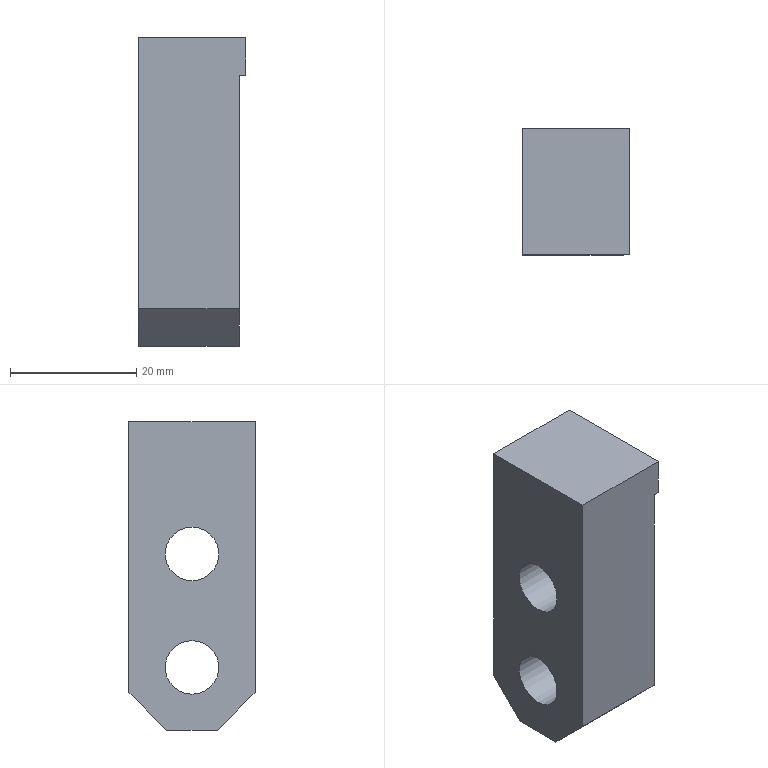Part | STEP file | gslz 2016.10.28-13_id1622_x_t | 1 solid | 16 faces | box 17 x 20 x 49 mm | volume 11659 mm3 | plane 12 | cylinder 4 | commonest cylinder face diameters 8.5 x2 14 x2
STEP:
#1=CARTESIAN_POINT('',(0.,0.,0.));
#2=DIRECTION('',(0.,0.,1.));
#3=DIRECTION('',(1.,0.,0.));
#4=AXIS2_PLACEMENT_3D('',#1,#2,#3);
#5=CARTESIAN_POINT('',(1326.873,56.996,-43.));
#6=VERTEX_POINT('',#5);
#7=CARTESIAN_POINT('',(1326.873,56.996,-6.));
#8=VERTEX_POINT('',#7);
#9=CARTESIAN_POINT('',(1326.873,56.996,-30.));
#10=DIRECTION('',(0.,0.,1.));
#11=VECTOR('',#10,1.);
#12=LINE('',#9,#11);
#13=CARTESIAN_POINT('',(1327.873,56.996,-30.));
#14=DIRECTION('',(0.,-1.,0.));
#15=DIRECTION('',(0.,0.,-1.));
#16=AXIS2_PLACEMENT_3D('',#13,#14,#15);
#17=PLANE('',#16);
#18=CARTESIAN_POINT('',(0.,-1.));
#19=DIRECTION('',(-1.,0.));
#20=VECTOR('',#19,1.);
#21=LINE('',#18,#20);
#22=(GEOMETRIC_REPRESENTATION_CONTEXT(2)PARAMETRIC_REPRESENTATION_CONTEXT()REPRESENTATION_CONTEXT('',''));
#23=DEFINITIONAL_REPRESENTATION('',(#21),#22);
#24=PCURVE('',#17,#23);
#25=CARTESIAN_POINT('',(1326.873,1026.996,-30.));
#26=DIRECTION('',(-1.,0.,0.));
#27=DIRECTION('',(0.,0.,1.));
#28=AXIS2_PLACEMENT_3D('',#25,#26,#27);
#29=PLANE('',#28);
#30=CARTESIAN_POINT('',(0.,-970.));
#31=DIRECTION('',(1.,0.));
#32=VECTOR('',#31,1.);
#33=LINE('',#30,#32);
#34=(GEOMETRIC_REPRESENTATION_CONTEXT(2)PARAMETRIC_REPRESENTATION_CONTEXT()REPRESENTATION_CONTEXT('',''));
#35=DEFINITIONAL_REPRESENTATION('',(#33),#34);
#36=PCURVE('',#29,#35);
#37=SURFACE_CURVE('',#12,(#24,#36),.PCURVE_S1.);
#38=EDGE_CURVE('',#6,#8,#37,.T.);
#39=ORIENTED_EDGE('',*,*,#38,.T.);
#40=CARTESIAN_POINT('',(1327.873,56.996,-6.));
#41=VERTEX_POINT('',#40);
#42=CARTESIAN_POINT('',(1327.873,56.996,-6.));
#43=DIRECTION('',(-1.,0.,0.));
#44=VECTOR('',#43,1.);
#45=LINE('',#42,#44);
#46=CARTESIAN_POINT('',(-24.,0.));
#47=DIRECTION('',(0.,-1.));
#48=VECTOR('',#47,1.);
#49=LINE('',#46,#48);
#50=(GEOMETRIC_REPRESENTATION_CONTEXT(2)PARAMETRIC_REPRESENTATION_CONTEXT()REPRESENTATION_CONTEXT('',''));
#51=DEFINITIONAL_REPRESENTATION('',(#49),#50);
#52=PCURVE('',#17,#51);
#53=CARTESIAN_POINT('',(1319.373,66.996,-6.));
#54=DIRECTION('',(0.,0.,1.));
#55=DIRECTION('',(1.,0.,0.));
#56=AXIS2_PLACEMENT_3D('',#53,#54,#55);
#57=PLANE('',#56);
#58=CARTESIAN_POINT('',(8.5,-10.));
#59=DIRECTION('',(-1.,0.));
#60=VECTOR('',#59,1.);
#61=LINE('',#58,#60);
#62=(GEOMETRIC_REPRESENTATION_CONTEXT(2)PARAMETRIC_REPRESENTATION_CONTEXT()REPRESENTATION_CONTEXT('',''));
#63=DEFINITIONAL_REPRESENTATION('',(#61),#62);
#64=PCURVE('',#57,#63);
#65=SURFACE_CURVE('',#45,(#52,#64),.PCURVE_S1.);
#66=EDGE_CURVE('',#41,#8,#65,.T.);
#67=ORIENTED_EDGE('',*,*,#66,.F.);
#68=CARTESIAN_POINT('',(1327.873,56.996,0.));
#69=VERTEX_POINT('',#68);
#70=CARTESIAN_POINT('',(1327.873,56.996,-30.));
#71=DIRECTION('',(0.,0.,1.));
#72=VECTOR('',#71,1.);
#73=LINE('',#70,#72);
#74=CARTESIAN_POINT('',(0.,0.));
#75=DIRECTION('',(-1.,0.));
#76=VECTOR('',#75,1.);
#77=LINE('',#74,#76);
#78=(GEOMETRIC_REPRESENTATION_CONTEXT(2)PARAMETRIC_REPRESENTATION_CONTEXT()REPRESENTATION_CONTEXT('',''));
#79=DEFINITIONAL_REPRESENTATION('',(#77),#78);
#80=PCURVE('',#17,#79);
#81=CARTESIAN_POINT('',(1327.873,1026.996,-30.));
#82=DIRECTION('',(-1.,0.,0.));
#83=DIRECTION('',(0.,0.,1.));
#84=AXIS2_PLACEMENT_3D('',#81,#82,#83);
#85=PLANE('',#84);
#86=CARTESIAN_POINT('',(0.,-970.));
#87=DIRECTION('',(1.,0.));
#88=VECTOR('',#87,1.);
#89=LINE('',#86,#88);
#90=(GEOMETRIC_REPRESENTATION_CONTEXT(2)PARAMETRIC_REPRESENTATION_CONTEXT()REPRESENTATION_CONTEXT('',''));
#91=DEFINITIONAL_REPRESENTATION('',(#89),#90);
#92=PCURVE('',#85,#91);
#93=SURFACE_CURVE('',#73,(#80,#92),.PCURVE_S1.);
#94=EDGE_CURVE('',#41,#69,#93,.T.);
#95=ORIENTED_EDGE('',*,*,#94,.T.);
#96=CARTESIAN_POINT('',(1310.873,56.996,0.));
#97=VERTEX_POINT('',#96);
#98=CARTESIAN_POINT('',(1327.873,56.996,0.));
#99=DIRECTION('',(-1.,0.,0.));
#100=VECTOR('',#99,1.);
#101=LINE('',#98,#100);
#102=CARTESIAN_POINT('',(-30.,0.));
#103=DIRECTION('',(0.,-1.));
#104=VECTOR('',#103,1.);
#105=LINE('',#102,#104);
#106=(GEOMETRIC_REPRESENTATION_CONTEXT(2)PARAMETRIC_REPRESENTATION_CONTEXT()REPRESENTATION_CONTEXT('',''));
#107=DEFINITIONAL_REPRESENTATION('',(#105),#106);
#108=PCURVE('',#17,#107);
#109=CARTESIAN_POINT('',(1254.028,32.871,0.));
#110=DIRECTION('',(0.,0.,1.));
#111=DIRECTION('',(1.,0.,0.));
#112=AXIS2_PLACEMENT_3D('',#109,#110,#111);
#113=PLANE('',#112);
#114=CARTESIAN_POINT('',(73.845,24.125));
#115=DIRECTION('',(-1.,0.));
#116=VECTOR('',#115,1.);
#117=LINE('',#114,#116);
#118=(GEOMETRIC_REPRESENTATION_CONTEXT(2)PARAMETRIC_REPRESENTATION_CONTEXT()REPRESENTATION_CONTEXT('',''));
#119=DEFINITIONAL_REPRESENTATION('',(#117),#118);
#120=PCURVE('',#113,#119);
#121=SURFACE_CURVE('',#101,(#108,#120),.PCURVE_S1.);
#122=EDGE_CURVE('',#69,#97,#121,.T.);
#123=ORIENTED_EDGE('',*,*,#122,.T.);
#124=CARTESIAN_POINT('',(1310.873,56.996,-43.));
#125=VERTEX_POINT('',#124);
#126=CARTESIAN_POINT('',(1310.873,56.996,-30.));
#127=DIRECTION('',(0.,0.,-1.));
#128=VECTOR('',#127,1.);
#129=LINE('',#126,#128);
#130=CARTESIAN_POINT('',(0.,-17.));
#131=DIRECTION('',(1.,0.));
#132=VECTOR('',#131,1.);
#133=LINE('',#130,#132);
#134=(GEOMETRIC_REPRESENTATION_CONTEXT(2)PARAMETRIC_REPRESENTATION_CONTEXT()REPRESENTATION_CONTEXT('',''));
#135=DEFINITIONAL_REPRESENTATION('',(#133),#134);
#136=PCURVE('',#17,#135);
#137=CARTESIAN_POINT('',(1310.873,1026.996,-30.));
#138=DIRECTION('',(-1.,0.,0.));
#139=DIRECTION('',(0.,0.,1.));
#140=AXIS2_PLACEMENT_3D('',#137,#138,#139);
#141=PLANE('',#140);
#142=CARTESIAN_POINT('',(0.,-970.));
#143=DIRECTION('',(-1.,0.));
#144=VECTOR('',#143,1.);
#145=LINE('',#142,#144);
#146=(GEOMETRIC_REPRESENTATION_CONTEXT(2)PARAMETRIC_REPRESENTATION_CONTEXT()REPRESENTATION_CONTEXT('',''));
#147=DEFINITIONAL_REPRESENTATION('',(#145),#146);
#148=PCURVE('',#141,#147);
#149=SURFACE_CURVE('',#129,(#136,#148),.PCURVE_S1.);
#150=EDGE_CURVE('',#97,#125,#149,.T.);
#151=ORIENTED_EDGE('',*,*,#150,.T.);
#152=CARTESIAN_POINT('',(1327.873,56.996,-43.));
#153=DIRECTION('',(1.,0.,0.));
#154=VECTOR('',#153,1.);
#155=LINE('',#152,#154);
#156=CARTESIAN_POINT('',(13.,0.));
#157=DIRECTION('',(0.,1.));
#158=VECTOR('',#157,1.);
#159=LINE('',#156,#158);
#160=(GEOMETRIC_REPRESENTATION_CONTEXT(2)PARAMETRIC_REPRESENTATION_CONTEXT()REPRESENTATION_CONTEXT('',''));
#161=DEFINITIONAL_REPRESENTATION('',(#159),#160);
#162=PCURVE('',#17,#161);
#163=CARTESIAN_POINT('',(-312.318,62.996,-49.));
#164=DIRECTION('',(0.,-0.7071,-0.7071));
#165=DIRECTION('',(1.,0.,0.));
#166=AXIS2_PLACEMENT_3D('',#163,#164,#165);
#167=PLANE('',#166);
#168=CARTESIAN_POINT('',(1640.191,8.485));
#169=DIRECTION('',(1.,0.));
#170=VECTOR('',#169,1.);
#171=LINE('',#168,#170);
#172=(GEOMETRIC_REPRESENTATION_CONTEXT(2)PARAMETRIC_REPRESENTATION_CONTEXT()REPRESENTATION_CONTEXT('',''));
#173=DEFINITIONAL_REPRESENTATION('',(#171),#172);
#174=PCURVE('',#167,#173);
#175=SURFACE_CURVE('',#155,(#162,#174),.PCURVE_S1.);
#176=EDGE_CURVE('',#125,#6,#175,.T.);
#177=ORIENTED_EDGE('',*,*,#176,.T.);
#178=EDGE_LOOP('',(#39,#67,#95,#123,#151,#177));
#179=FACE_BOUND('',#178,.T.);
#180=ADVANCED_FACE('',(#179),#17,.T.);
#181=CARTESIAN_POINT('',(1310.873,76.996,-43.));
#182=VERTEX_POINT('',#181);
#183=CARTESIAN_POINT('',(1310.873,76.996,0.));
#184=VERTEX_POINT('',#183);
#185=CARTESIAN_POINT('',(1310.873,76.996,-30.));
#186=DIRECTION('',(0.,0.,1.));
#187=VECTOR('',#186,1.);
#188=LINE('',#185,#187);
#189=CARTESIAN_POINT('',(1302.873,76.996,-79.));
#190=DIRECTION('',(0.,1.,0.));
#191=DIRECTION('',(0.,0.,1.));
#192=AXIS2_PLACEMENT_3D('',#189,#190,#191);
#193=PLANE('',#192);
#194=CARTESIAN_POINT('',(49.,8.));
#195=DIRECTION('',(1.,0.));
#196=VECTOR('',#195,1.);
#197=LINE('',#194,#196);
#198=(GEOMETRIC_REPRESENTATION_CONTEXT(2)PARAMETRIC_REPRESENTATION_CONTEXT()REPRESENTATION_CONTEXT('',''));
#199=DEFINITIONAL_REPRESENTATION('',(#197),#198);
#200=PCURVE('',#193,#199);
#201=CARTESIAN_POINT('',(0.,-950.));
#202=DIRECTION('',(1.,0.));
#203=VECTOR('',#202,1.);
#204=LINE('',#201,#203);
#205=(GEOMETRIC_REPRESENTATION_CONTEXT(2)PARAMETRIC_REPRESENTATION_CONTEXT()REPRESENTATION_CONTEXT('',''));
#206=DEFINITIONAL_REPRESENTATION('',(#204),#205);
#207=PCURVE('',#141,#206);
#208=SURFACE_CURVE('',#188,(#200,#207),.PCURVE_S1.);
#209=EDGE_CURVE('',#182,#184,#208,.T.);
#210=ORIENTED_EDGE('',*,*,#209,.T.);
#211=CARTESIAN_POINT('',(1327.873,76.996,0.));
#212=VERTEX_POINT('',#211);
#213=CARTESIAN_POINT('',(1254.028,76.996,0.));
#214=DIRECTION('',(-1.,0.,0.));
#215=VECTOR('',#214,1.);
#216=LINE('',#213,#215);
#217=CARTESIAN_POINT('',(79.,-48.845));
#218=DIRECTION('',(0.,-1.));
#219=VECTOR('',#218,1.);
#220=LINE('',#217,#219);
#221=(GEOMETRIC_REPRESENTATION_CONTEXT(2)PARAMETRIC_REPRESENTATION_CONTEXT()REPRESENTATION_CONTEXT('',''));
#222=DEFINITIONAL_REPRESENTATION('',(#220),#221);
#223=PCURVE('',#193,#222);
#224=CARTESIAN_POINT('',(0.,44.125));
#225=DIRECTION('',(-1.,0.));
#226=VECTOR('',#225,1.);
#227=LINE('',#224,#226);
#228=(GEOMETRIC_REPRESENTATION_CONTEXT(2)PARAMETRIC_REPRESENTATION_CONTEXT()REPRESENTATION_CONTEXT('',''));
#229=DEFINITIONAL_REPRESENTATION('',(#227),#228);
#230=PCURVE('',#113,#229);
#231=SURFACE_CURVE('',#216,(#223,#230),.PCURVE_S1.);
#232=EDGE_CURVE('',#212,#184,#231,.T.);
#233=ORIENTED_EDGE('',*,*,#232,.F.);
#234=CARTESIAN_POINT('',(1327.873,76.996,-6.));
#235=VERTEX_POINT('',#234);
#236=CARTESIAN_POINT('',(1327.873,76.996,-30.));
#237=DIRECTION('',(0.,0.,-1.));
#238=VECTOR('',#237,1.);
#239=LINE('',#236,#238);
#240=CARTESIAN_POINT('',(49.,25.));
#241=DIRECTION('',(-1.,0.));
#242=VECTOR('',#241,1.);
#243=LINE('',#240,#242);
#244=(GEOMETRIC_REPRESENTATION_CONTEXT(2)PARAMETRIC_REPRESENTATION_CONTEXT()REPRESENTATION_CONTEXT('',''));
#245=DEFINITIONAL_REPRESENTATION('',(#243),#244);
#246=PCURVE('',#193,#245);
#247=CARTESIAN_POINT('',(0.,-950.));
#248=DIRECTION('',(-1.,0.));
#249=VECTOR('',#248,1.);
#250=LINE('',#247,#249);
#251=(GEOMETRIC_REPRESENTATION_CONTEXT(2)PARAMETRIC_REPRESENTATION_CONTEXT()REPRESENTATION_CONTEXT('',''));
#252=DEFINITIONAL_REPRESENTATION('',(#250),#251);
#253=PCURVE('',#85,#252);
#254=SURFACE_CURVE('',#239,(#246,#253),.PCURVE_S1.);
#255=EDGE_CURVE('',#212,#235,#254,.T.);
#256=ORIENTED_EDGE('',*,*,#255,.T.);
#257=CARTESIAN_POINT('',(1326.873,76.996,-6.));
#258=VERTEX_POINT('',#257);
#259=CARTESIAN_POINT('',(1302.873,76.996,-6.));
#260=DIRECTION('',(1.,0.,0.));
#261=VECTOR('',#260,1.);
#262=LINE('',#259,#261);
#263=CARTESIAN_POINT('',(73.,0.));
#264=DIRECTION('',(0.,1.));
#265=VECTOR('',#264,1.);
#266=LINE('',#263,#265);
#267=(GEOMETRIC_REPRESENTATION_CONTEXT(2)PARAMETRIC_REPRESENTATION_CONTEXT()REPRESENTATION_CONTEXT('',''));
#268=DEFINITIONAL_REPRESENTATION('',(#266),#267);
#269=PCURVE('',#193,#268);
#270=CARTESIAN_POINT('',(-16.5,10.));
#271=DIRECTION('',(1.,0.));
#272=VECTOR('',#271,1.);
#273=LINE('',#270,#272);
#274=(GEOMETRIC_REPRESENTATION_CONTEXT(2)PARAMETRIC_REPRESENTATION_CONTEXT()REPRESENTATION_CONTEXT('',''));
#275=DEFINITIONAL_REPRESENTATION('',(#273),#274);
#276=PCURVE('',#57,#275);
#277=SURFACE_CURVE('',#262,(#269,#276),.PCURVE_S1.);
#278=EDGE_CURVE('',#258,#235,#277,.T.);
#279=ORIENTED_EDGE('',*,*,#278,.F.);
#280=CARTESIAN_POINT('',(1326.873,76.996,-43.));
#281=VERTEX_POINT('',#280);
#282=CARTESIAN_POINT('',(1326.873,76.996,-30.));
#283=DIRECTION('',(0.,0.,-1.));
#284=VECTOR('',#283,1.);
#285=LINE('',#282,#284);
#286=CARTESIAN_POINT('',(49.,24.));
#287=DIRECTION('',(-1.,0.));
#288=VECTOR('',#287,1.);
#289=LINE('',#286,#288);
#290=(GEOMETRIC_REPRESENTATION_CONTEXT(2)PARAMETRIC_REPRESENTATION_CONTEXT()REPRESENTATION_CONTEXT('',''));
#291=DEFINITIONAL_REPRESENTATION('',(#289),#290);
#292=PCURVE('',#193,#291);
#293=CARTESIAN_POINT('',(0.,-950.));
#294=DIRECTION('',(-1.,0.));
#295=VECTOR('',#294,1.);
#296=LINE('',#293,#295);
#297=(GEOMETRIC_REPRESENTATION_CONTEXT(2)PARAMETRIC_REPRESENTATION_CONTEXT()REPRESENTATION_CONTEXT('',''));
#298=DEFINITIONAL_REPRESENTATION('',(#296),#297);
#299=PCURVE('',#29,#298);
#300=SURFACE_CURVE('',#285,(#292,#299),.PCURVE_S1.);
#301=EDGE_CURVE('',#258,#281,#300,.T.);
#302=ORIENTED_EDGE('',*,*,#301,.T.);
#303=CARTESIAN_POINT('',(1302.873,76.996,-43.));
#304=DIRECTION('',(-1.,0.,0.));
#305=VECTOR('',#304,1.);
#306=LINE('',#303,#305);
#307=CARTESIAN_POINT('',(36.,0.));
#308=DIRECTION('',(0.,-1.));
#309=VECTOR('',#308,1.);
#310=LINE('',#307,#309);
#311=(GEOMETRIC_REPRESENTATION_CONTEXT(2)PARAMETRIC_REPRESENTATION_CONTEXT()REPRESENTATION_CONTEXT('',''));
#312=DEFINITIONAL_REPRESENTATION('',(#310),#311);
#313=PCURVE('',#193,#312);
#314=CARTESIAN_POINT('',(1302.873,76.996,-43.));
#315=DIRECTION('',(0.,0.7071,-0.7071));
#316=DIRECTION('',(1.,0.,0.));
#317=AXIS2_PLACEMENT_3D('',#314,#315,#316);
#318=PLANE('',#317);
#319=CARTESIAN_POINT('',(0.,0.));
#320=DIRECTION('',(-1.,0.));
#321=VECTOR('',#320,1.);
#322=LINE('',#319,#321);
#323=(GEOMETRIC_REPRESENTATION_CONTEXT(2)PARAMETRIC_REPRESENTATION_CONTEXT()REPRESENTATION_CONTEXT('',''));
#324=DEFINITIONAL_REPRESENTATION('',(#322),#323);
#325=PCURVE('',#318,#324);
#326=SURFACE_CURVE('',#306,(#313,#325),.PCURVE_S1.);
#327=EDGE_CURVE('',#281,#182,#326,.T.);
#328=ORIENTED_EDGE('',*,*,#327,.T.);
#329=EDGE_LOOP('',(#210,#233,#256,#279,#302,#328));
#330=FACE_BOUND('',#329,.T.);
#331=ADVANCED_FACE('',(#330),#193,.T.);
#332=CARTESIAN_POINT('',(1310.873,66.996,-34.75));
#333=VERTEX_POINT('',#332);
#334=CARTESIAN_POINT('',(1310.873,66.996,-39.));
#335=DIRECTION('',(1.,0.,0.));
#336=DIRECTION('',(0.,0.,1.));
#337=AXIS2_PLACEMENT_3D('',#334,#335,#336);
#338=CIRCLE('',#337,4.25);
#339=CARTESIAN_POINT('',(-4.75,-960.));
#340=CARTESIAN_POINT('',(-4.75,-967.361));
#341=CARTESIAN_POINT('',(-11.125,-963.681));
#342=CARTESIAN_POINT('',(-17.5,-960.));
#343=CARTESIAN_POINT('',(-11.125,-956.319));
#344=CARTESIAN_POINT('',(-4.75,-952.639));
#345=CARTESIAN_POINT('',(-4.75,-960.));
#346=(BOUNDED_CURVE()B_SPLINE_CURVE(2,(#339,#340,#341,#342,#343,#344,#345),.UNSPECIFIED.,.T.,.F.)B_SPLINE_CURVE_WITH_KNOTS((1,2,2,2,2,1),(-2.094,0.,2.094,4.189,6.283,8.378),.UNSPECIFIED.)CURVE()GEOMETRIC_REPRESENTATION_ITEM()RATIONAL_B_SPLINE_CURVE((1.,0.5,1.,0.5,1.,0.5,1.))REPRESENTATION_ITEM(''));
#347=(GEOMETRIC_REPRESENTATION_CONTEXT(2)PARAMETRIC_REPRESENTATION_CONTEXT()REPRESENTATION_CONTEXT('',''));
#348=DEFINITIONAL_REPRESENTATION('',(#346),#347);
#349=PCURVE('',#141,#348);
#350=CARTESIAN_POINT('',(1277.873,66.996,-39.));
#351=DIRECTION('',(-1.,0.,0.));
#352=DIRECTION('',(0.,0.,1.));
#353=AXIS2_PLACEMENT_3D('',#350,#351,#352);
#354=CYLINDRICAL_SURFACE('',#353,4.25);
#355=CARTESIAN_POINT('',(6.283,-33.));
#356=DIRECTION('',(-1.,0.));
#357=VECTOR('',#356,1.);
#358=LINE('',#355,#357);
#359=(GEOMETRIC_REPRESENTATION_CONTEXT(2)PARAMETRIC_REPRESENTATION_CONTEXT()REPRESENTATION_CONTEXT('',''));
#360=DEFINITIONAL_REPRESENTATION('',(#358),#359);
#361=PCURVE('',#354,#360);
#362=SURFACE_CURVE('',#338,(#349,#361),.PCURVE_S1.);
#363=EDGE_CURVE('',#333,#333,#362,.T.);
#364=ORIENTED_EDGE('',*,*,#363,.T.);
#365=EDGE_LOOP('',(#364));
#366=FACE_BOUND('',#365,.T.);
#367=CARTESIAN_POINT('',(1310.873,66.996,-16.75));
#368=VERTEX_POINT('',#367);
#369=CARTESIAN_POINT('',(1310.873,66.996,-21.));
#370=DIRECTION('',(1.,0.,0.));
#371=DIRECTION('',(0.,0.,1.));
#372=AXIS2_PLACEMENT_3D('',#369,#370,#371);
#373=CIRCLE('',#372,4.25);
#374=CARTESIAN_POINT('',(13.25,-960.));
#375=CARTESIAN_POINT('',(13.25,-967.361));
#376=CARTESIAN_POINT('',(6.875,-963.681));
#377=CARTESIAN_POINT('',(0.5,-960.));
#378=CARTESIAN_POINT('',(6.875,-956.319));
#379=CARTESIAN_POINT('',(13.25,-952.639));
#380=CARTESIAN_POINT('',(13.25,-960.));
#381=(BOUNDED_CURVE()B_SPLINE_CURVE(2,(#374,#375,#376,#377,#378,#379,#380),.UNSPECIFIED.,.T.,.F.)B_SPLINE_CURVE_WITH_KNOTS((1,2,2,2,2,1),(-2.094,0.,2.094,4.189,6.283,8.378),.UNSPECIFIED.)CURVE()GEOMETRIC_REPRESENTATION_ITEM()RATIONAL_B_SPLINE_CURVE((1.,0.5,1.,0.5,1.,0.5,1.))REPRESENTATION_ITEM(''));
#382=(GEOMETRIC_REPRESENTATION_CONTEXT(2)PARAMETRIC_REPRESENTATION_CONTEXT()REPRESENTATION_CONTEXT('',''));
#383=DEFINITIONAL_REPRESENTATION('',(#381),#382);
#384=PCURVE('',#141,#383);
#385=CARTESIAN_POINT('',(1277.873,66.996,-21.));
#386=DIRECTION('',(-1.,0.,0.));
#387=DIRECTION('',(0.,0.,1.));
#388=AXIS2_PLACEMENT_3D('',#385,#386,#387);
#389=CYLINDRICAL_SURFACE('',#388,4.25);
#390=CARTESIAN_POINT('',(6.283,-33.));
#391=DIRECTION('',(-1.,0.));
#392=VECTOR('',#391,1.);
#393=LINE('',#390,#392);
#394=(GEOMETRIC_REPRESENTATION_CONTEXT(2)PARAMETRIC_REPRESENTATION_CONTEXT()REPRESENTATION_CONTEXT('',''));
#395=DEFINITIONAL_REPRESENTATION('',(#393),#394);
#396=PCURVE('',#389,#395);
#397=SURFACE_CURVE('',#373,(#384,#396),.PCURVE_S1.);
#398=EDGE_CURVE('',#368,#368,#397,.T.);
#399=ORIENTED_EDGE('',*,*,#398,.T.);
#400=EDGE_LOOP('',(#399));
#401=FACE_BOUND('',#400,.T.);
#402=ORIENTED_EDGE('',*,*,#150,.F.);
#403=CARTESIAN_POINT('',(1310.873,1026.996,0.));
#404=DIRECTION('',(0.,-1.,0.));
#405=VECTOR('',#404,1.);
#406=LINE('',#403,#405);
#407=CARTESIAN_POINT('',(30.,0.));
#408=DIRECTION('',(0.,-1.));
#409=VECTOR('',#408,1.);
#410=LINE('',#407,#409);
#411=(GEOMETRIC_REPRESENTATION_CONTEXT(2)PARAMETRIC_REPRESENTATION_CONTEXT()REPRESENTATION_CONTEXT('',''));
#412=DEFINITIONAL_REPRESENTATION('',(#410),#411);
#413=PCURVE('',#141,#412);
#414=CARTESIAN_POINT('',(56.845,994.125));
#415=DIRECTION('',(0.,-1.));
#416=VECTOR('',#415,1.);
#417=LINE('',#414,#416);
#418=(GEOMETRIC_REPRESENTATION_CONTEXT(2)PARAMETRIC_REPRESENTATION_CONTEXT()REPRESENTATION_CONTEXT('',''));
#419=DEFINITIONAL_REPRESENTATION('',(#417),#418);
#420=PCURVE('',#113,#419);
#421=SURFACE_CURVE('',#406,(#413,#420),.PCURVE_S1.);
#422=EDGE_CURVE('',#184,#97,#421,.T.);
#423=ORIENTED_EDGE('',*,*,#422,.F.);
#424=ORIENTED_EDGE('',*,*,#209,.F.);
#425=CARTESIAN_POINT('',(1310.873,70.996,-49.));
#426=VERTEX_POINT('',#425);
#427=CARTESIAN_POINT('',(1310.873,76.996,-43.));
#428=DIRECTION('',(0.,-0.7071,-0.7071));
#429=VECTOR('',#428,1.);
#430=LINE('',#427,#429);
#431=CARTESIAN_POINT('',(-13.,-950.));
#432=DIRECTION('',(-0.7071,-0.7071));
#433=VECTOR('',#432,1.);
#434=LINE('',#431,#433);
#435=(GEOMETRIC_REPRESENTATION_CONTEXT(2)PARAMETRIC_REPRESENTATION_CONTEXT()REPRESENTATION_CONTEXT('',''));
#436=DEFINITIONAL_REPRESENTATION('',(#434),#435);
#437=PCURVE('',#141,#436);
#438=CARTESIAN_POINT('',(8.,0.));
#439=DIRECTION('',(0.,1.));
#440=VECTOR('',#439,1.);
#441=LINE('',#438,#440);
#442=(GEOMETRIC_REPRESENTATION_CONTEXT(2)PARAMETRIC_REPRESENTATION_CONTEXT()REPRESENTATION_CONTEXT('',''));
#443=DEFINITIONAL_REPRESENTATION('',(#441),#442);
#444=PCURVE('',#318,#443);
#445=SURFACE_CURVE('',#430,(#437,#444),.PCURVE_S1.);
#446=EDGE_CURVE('',#182,#426,#445,.T.);
#447=ORIENTED_EDGE('',*,*,#446,.T.);
#448=CARTESIAN_POINT('',(1310.873,62.996,-49.));
#449=VERTEX_POINT('',#448);
#450=CARTESIAN_POINT('',(1310.873,1026.996,-49.));
#451=DIRECTION('',(0.,1.,0.));
#452=VECTOR('',#451,1.);
#453=LINE('',#450,#452);
#454=CARTESIAN_POINT('',(-19.,0.));
#455=DIRECTION('',(0.,1.));
#456=VECTOR('',#455,1.);
#457=LINE('',#454,#456);
#458=(GEOMETRIC_REPRESENTATION_CONTEXT(2)PARAMETRIC_REPRESENTATION_CONTEXT()REPRESENTATION_CONTEXT('',''));
#459=DEFINITIONAL_REPRESENTATION('',(#457),#458);
#460=PCURVE('',#141,#459);
#461=CARTESIAN_POINT('',(-312.318,-6.022,-49.));
#462=DIRECTION('',(0.,0.,1.));
#463=DIRECTION('',(1.,0.,0.));
#464=AXIS2_PLACEMENT_3D('',#461,#462,#463);
#465=PLANE('',#464);
#466=CARTESIAN_POINT('',(1623.191,1033.018));
#467=DIRECTION('',(0.,1.));
#468=VECTOR('',#467,1.);
#469=LINE('',#466,#468);
#470=(GEOMETRIC_REPRESENTATION_CONTEXT(2)PARAMETRIC_REPRESENTATION_CONTEXT()REPRESENTATION_CONTEXT('',''));
#471=DEFINITIONAL_REPRESENTATION('',(#469),#470);
#472=PCURVE('',#465,#471);
#473=SURFACE_CURVE('',#453,(#460,#472),.PCURVE_S1.);
#474=EDGE_CURVE('',#449,#426,#473,.T.);
#475=ORIENTED_EDGE('',*,*,#474,.F.);
#476=CARTESIAN_POINT('',(1310.873,62.996,-49.));
#477=DIRECTION('',(0.,-0.7071,0.7071));
#478=VECTOR('',#477,1.);
#479=LINE('',#476,#478);
#480=CARTESIAN_POINT('',(-19.,-964.));
#481=DIRECTION('',(0.7071,-0.7071));
#482=VECTOR('',#481,1.);
#483=LINE('',#480,#482);
#484=(GEOMETRIC_REPRESENTATION_CONTEXT(2)PARAMETRIC_REPRESENTATION_CONTEXT()REPRESENTATION_CONTEXT('',''));
#485=DEFINITIONAL_REPRESENTATION('',(#483),#484);
#486=PCURVE('',#141,#485);
#487=CARTESIAN_POINT('',(1623.191,0.));
#488=DIRECTION('',(0.,1.));
#489=VECTOR('',#488,1.);
#490=LINE('',#487,#489);
#491=(GEOMETRIC_REPRESENTATION_CONTEXT(2)PARAMETRIC_REPRESENTATION_CONTEXT()REPRESENTATION_CONTEXT('',''));
#492=DEFINITIONAL_REPRESENTATION('',(#490),#491);
#493=PCURVE('',#167,#492);
#494=SURFACE_CURVE('',#479,(#486,#493),.PCURVE_S1.);
#495=EDGE_CURVE('',#449,#125,#494,.T.);
#496=ORIENTED_EDGE('',*,*,#495,.T.);
#497=EDGE_LOOP('',(#402,#423,#424,#447,#475,#496));
#498=FACE_BOUND('',#497,.T.);
#499=ADVANCED_FACE('',(#366,#401,#498),#141,.T.);
#500=CARTESIAN_POINT('',(1326.873,66.996,-32.));
#501=VERTEX_POINT('',#500);
#502=CARTESIAN_POINT('',(1326.873,66.996,-39.));
#503=DIRECTION('',(-1.,0.,0.));
#504=DIRECTION('',(0.,0.,1.));
#505=AXIS2_PLACEMENT_3D('',#502,#503,#504);
#506=CIRCLE('',#505,7.);
#507=CARTESIAN_POINT('',(-9.,-960.));
#508=DIRECTION('',(1.,0.));
#509=AXIS2_PLACEMENT_2D('',#507,#508);
#510=CIRCLE('',#509,7.);
#511=(GEOMETRIC_REPRESENTATION_CONTEXT(2)PARAMETRIC_REPRESENTATION_CONTEXT()REPRESENTATION_CONTEXT('',''));
#512=DEFINITIONAL_REPRESENTATION('',(#510),#511);
#513=PCURVE('',#29,#512);
#514=CARTESIAN_POINT('',(1327.873,66.996,-39.));
#515=DIRECTION('',(-1.,0.,0.));
#516=DIRECTION('',(0.,0.,1.));
#517=AXIS2_PLACEMENT_3D('',#514,#515,#516);
#518=CYLINDRICAL_SURFACE('',#517,7.);
#519=CARTESIAN_POINT('',(0.,1.));
#520=DIRECTION('',(1.,0.));
#521=VECTOR('',#520,1.);
#522=LINE('',#519,#521);
#523=(GEOMETRIC_REPRESENTATION_CONTEXT(2)PARAMETRIC_REPRESENTATION_CONTEXT()REPRESENTATION_CONTEXT('',''));
#524=DEFINITIONAL_REPRESENTATION('',(#522),#523);
#525=PCURVE('',#518,#524);
#526=SURFACE_CURVE('',#506,(#513,#525),.PCURVE_S1.);
#527=EDGE_CURVE('',#501,#501,#526,.T.);
#528=ORIENTED_EDGE('',*,*,#527,.T.);
#529=EDGE_LOOP('',(#528));
#530=FACE_BOUND('',#529,.T.);
#531=CARTESIAN_POINT('',(1326.873,66.996,-14.));
#532=VERTEX_POINT('',#531);
#533=CARTESIAN_POINT('',(1326.873,66.996,-21.));
#534=DIRECTION('',(-1.,0.,0.));
#535=DIRECTION('',(0.,0.,1.));
#536=AXIS2_PLACEMENT_3D('',#533,#534,#535);
#537=CIRCLE('',#536,7.);
#538=CARTESIAN_POINT('',(9.,-960.));
#539=DIRECTION('',(1.,0.));
#540=AXIS2_PLACEMENT_2D('',#538,#539);
#541=CIRCLE('',#540,7.);
#542=(GEOMETRIC_REPRESENTATION_CONTEXT(2)PARAMETRIC_REPRESENTATION_CONTEXT()REPRESENTATION_CONTEXT('',''));
#543=DEFINITIONAL_REPRESENTATION('',(#541),#542);
#544=PCURVE('',#29,#543);
#545=CARTESIAN_POINT('',(1327.873,66.996,-21.));
#546=DIRECTION('',(-1.,0.,0.));
#547=DIRECTION('',(0.,0.,1.));
#548=AXIS2_PLACEMENT_3D('',#545,#546,#547);
#549=CYLINDRICAL_SURFACE('',#548,7.);
#550=CARTESIAN_POINT('',(0.,1.));
#551=DIRECTION('',(1.,0.));
#552=VECTOR('',#551,1.);
#553=LINE('',#550,#552);
#554=(GEOMETRIC_REPRESENTATION_CONTEXT(2)PARAMETRIC_REPRESENTATION_CONTEXT()REPRESENTATION_CONTEXT('',''));
#555=DEFINITIONAL_REPRESENTATION('',(#553),#554);
#556=PCURVE('',#549,#555);
#557=SURFACE_CURVE('',#537,(#544,#556),.PCURVE_S1.);
#558=EDGE_CURVE('',#532,#532,#557,.T.);
#559=ORIENTED_EDGE('',*,*,#558,.T.);
#560=EDGE_LOOP('',(#559));
#561=FACE_BOUND('',#560,.T.);
#562=CARTESIAN_POINT('',(1326.873,1026.996,-6.));
#563=DIRECTION('',(0.,-1.,0.));
#564=VECTOR('',#563,1.);
#565=LINE('',#562,#564);
#566=CARTESIAN_POINT('',(24.,0.));
#567=DIRECTION('',(0.,-1.));
#568=VECTOR('',#567,1.);
#569=LINE('',#566,#568);
#570=(GEOMETRIC_REPRESENTATION_CONTEXT(2)PARAMETRIC_REPRESENTATION_CONTEXT()REPRESENTATION_CONTEXT('',''));
#571=DEFINITIONAL_REPRESENTATION('',(#569),#570);
#572=PCURVE('',#29,#571);
#573=CARTESIAN_POINT('',(7.5,960.));
#574=DIRECTION('',(0.,-1.));
#575=VECTOR('',#574,1.);
#576=LINE('',#573,#575);
#577=(GEOMETRIC_REPRESENTATION_CONTEXT(2)PARAMETRIC_REPRESENTATION_CONTEXT()REPRESENTATION_CONTEXT('',''));
#578=DEFINITIONAL_REPRESENTATION('',(#576),#577);
#579=PCURVE('',#57,#578);
#580=SURFACE_CURVE('',#565,(#572,#579),.PCURVE_S1.);
#581=EDGE_CURVE('',#258,#8,#580,.T.);
#582=ORIENTED_EDGE('',*,*,#581,.T.);
#583=ORIENTED_EDGE('',*,*,#38,.F.);
#584=CARTESIAN_POINT('',(1326.873,62.996,-49.));
#585=VERTEX_POINT('',#584);
#586=CARTESIAN_POINT('',(1326.873,62.996,-49.));
#587=DIRECTION('',(0.,0.7071,-0.7071));
#588=VECTOR('',#587,1.);
#589=LINE('',#586,#588);
#590=CARTESIAN_POINT('',(-19.,-964.));
#591=DIRECTION('',(-0.7071,0.7071));
#592=VECTOR('',#591,1.);
#593=LINE('',#590,#592);
#594=(GEOMETRIC_REPRESENTATION_CONTEXT(2)PARAMETRIC_REPRESENTATION_CONTEXT()REPRESENTATION_CONTEXT('',''));
#595=DEFINITIONAL_REPRESENTATION('',(#593),#594);
#596=PCURVE('',#29,#595);
#597=CARTESIAN_POINT('',(1639.191,0.));
#598=DIRECTION('',(0.,-1.));
#599=VECTOR('',#598,1.);
#600=LINE('',#597,#599);
#601=(GEOMETRIC_REPRESENTATION_CONTEXT(2)PARAMETRIC_REPRESENTATION_CONTEXT()REPRESENTATION_CONTEXT('',''));
#602=DEFINITIONAL_REPRESENTATION('',(#600),#601);
#603=PCURVE('',#167,#602);
#604=SURFACE_CURVE('',#589,(#596,#603),.PCURVE_S1.);
#605=EDGE_CURVE('',#6,#585,#604,.T.);
#606=ORIENTED_EDGE('',*,*,#605,.T.);
#607=CARTESIAN_POINT('',(1326.873,70.996,-49.));
#608=VERTEX_POINT('',#607);
#609=CARTESIAN_POINT('',(1326.873,1026.996,-49.));
#610=DIRECTION('',(0.,-1.,0.));
#611=VECTOR('',#610,1.);
#612=LINE('',#609,#611);
#613=CARTESIAN_POINT('',(-19.,0.));
#614=DIRECTION('',(0.,-1.));
#615=VECTOR('',#614,1.);
#616=LINE('',#613,#615);
#617=(GEOMETRIC_REPRESENTATION_CONTEXT(2)PARAMETRIC_REPRESENTATION_CONTEXT()REPRESENTATION_CONTEXT('',''));
#618=DEFINITIONAL_REPRESENTATION('',(#616),#617);
#619=PCURVE('',#29,#618);
#620=CARTESIAN_POINT('',(1639.191,1033.018));
#621=DIRECTION('',(0.,-1.));
#622=VECTOR('',#621,1.);
#623=LINE('',#620,#622);
#624=(GEOMETRIC_REPRESENTATION_CONTEXT(2)PARAMETRIC_REPRESENTATION_CONTEXT()REPRESENTATION_CONTEXT('',''));
#625=DEFINITIONAL_REPRESENTATION('',(#623),#624);
#626=PCURVE('',#465,#625);
#627=SURFACE_CURVE('',#612,(#619,#626),.PCURVE_S1.);
#628=EDGE_CURVE('',#608,#585,#627,.T.);
#629=ORIENTED_EDGE('',*,*,#628,.F.);
#630=CARTESIAN_POINT('',(1326.873,76.996,-43.));
#631=DIRECTION('',(0.,0.7071,0.7071));
#632=VECTOR('',#631,1.);
#633=LINE('',#630,#632);
#634=CARTESIAN_POINT('',(-13.,-950.));
#635=DIRECTION('',(0.7071,0.7071));
#636=VECTOR('',#635,1.);
#637=LINE('',#634,#636);
#638=(GEOMETRIC_REPRESENTATION_CONTEXT(2)PARAMETRIC_REPRESENTATION_CONTEXT()REPRESENTATION_CONTEXT('',''));
#639=DEFINITIONAL_REPRESENTATION('',(#637),#638);
#640=PCURVE('',#29,#639);
#641=CARTESIAN_POINT('',(24.,0.));
#642=DIRECTION('',(0.,-1.));
#643=VECTOR('',#642,1.);
#644=LINE('',#641,#643);
#645=(GEOMETRIC_REPRESENTATION_CONTEXT(2)PARAMETRIC_REPRESENTATION_CONTEXT()REPRESENTATION_CONTEXT('',''));
#646=DEFINITIONAL_REPRESENTATION('',(#644),#645);
#647=PCURVE('',#318,#646);
#648=SURFACE_CURVE('',#633,(#640,#647),.PCURVE_S1.);
#649=EDGE_CURVE('',#608,#281,#648,.T.);
#650=ORIENTED_EDGE('',*,*,#649,.T.);
#651=ORIENTED_EDGE('',*,*,#301,.F.);
#652=EDGE_LOOP('',(#582,#583,#606,#629,#650,#651));
#653=FACE_BOUND('',#652,.T.);
#654=ADVANCED_FACE('',(#530,#561,#653),#29,.F.);
#655=CARTESIAN_POINT('',(1317.873,66.996,-16.75));
#656=VERTEX_POINT('',#655);
#657=CARTESIAN_POINT('',(1317.873,66.996,-21.));
#658=DIRECTION('',(1.,0.,0.));
#659=DIRECTION('',(0.,0.,1.));
#660=AXIS2_PLACEMENT_3D('',#657,#658,#659);
#661=CIRCLE('',#660,4.25);
#662=CARTESIAN_POINT('',(1317.873,66.996,-21.));
#663=DIRECTION('',(-1.,0.,0.));
#664=DIRECTION('',(0.,0.,1.));
#665=AXIS2_PLACEMENT_3D('',#662,#663,#664);
#666=PLANE('',#665);
#667=CARTESIAN_POINT('',(4.25,0.));
#668=CARTESIAN_POINT('',(4.25,-7.361));
#669=CARTESIAN_POINT('',(-2.125,-3.681));
#670=CARTESIAN_POINT('',(-8.5,0.));
#671=CARTESIAN_POINT('',(-2.125,3.681));
#672=CARTESIAN_POINT('',(4.25,7.361));
#673=CARTESIAN_POINT('',(4.25,0.));
#674=(BOUNDED_CURVE()B_SPLINE_CURVE(2,(#667,#668,#669,#670,#671,#672,#673),.UNSPECIFIED.,.T.,.F.)B_SPLINE_CURVE_WITH_KNOTS((1,2,2,2,2,1),(-2.094,0.,2.094,4.189,6.283,8.378),.UNSPECIFIED.)CURVE()GEOMETRIC_REPRESENTATION_ITEM()RATIONAL_B_SPLINE_CURVE((1.,0.5,1.,0.5,1.,0.5,1.))REPRESENTATION_ITEM(''));
#675=(GEOMETRIC_REPRESENTATION_CONTEXT(2)PARAMETRIC_REPRESENTATION_CONTEXT()REPRESENTATION_CONTEXT('',''));
#676=DEFINITIONAL_REPRESENTATION('',(#674),#675);
#677=PCURVE('',#666,#676);
#678=CARTESIAN_POINT('',(6.283,-40.));
#679=DIRECTION('',(-1.,0.));
#680=VECTOR('',#679,1.);
#681=LINE('',#678,#680);
#682=(GEOMETRIC_REPRESENTATION_CONTEXT(2)PARAMETRIC_REPRESENTATION_CONTEXT()REPRESENTATION_CONTEXT('',''));
#683=DEFINITIONAL_REPRESENTATION('',(#681),#682);
#684=PCURVE('',#389,#683);
#685=SURFACE_CURVE('',#661,(#677,#684),.PCURVE_S1.);
#686=EDGE_CURVE('',#656,#656,#685,.T.);
#687=ORIENTED_EDGE('',*,*,#686,.F.);
#688=EDGE_LOOP('',(#687));
#689=FACE_BOUND('',#688,.T.);
#690=CARTESIAN_POINT('',(1317.873,66.996,-14.));
#691=VERTEX_POINT('',#690);
#692=CARTESIAN_POINT('',(1317.873,66.996,-21.));
#693=DIRECTION('',(1.,0.,0.));
#694=DIRECTION('',(0.,0.,1.));
#695=AXIS2_PLACEMENT_3D('',#692,#693,#694);
#696=CIRCLE('',#695,7.);
#697=CARTESIAN_POINT('',(7.,0.));
#698=CARTESIAN_POINT('',(7.,-12.124));
#699=CARTESIAN_POINT('',(-3.5,-6.062));
#700=CARTESIAN_POINT('',(-14.,0.));
#701=CARTESIAN_POINT('',(-3.5,6.062));
#702=CARTESIAN_POINT('',(7.,12.124));
#703=CARTESIAN_POINT('',(7.,0.));
#704=(BOUNDED_CURVE()B_SPLINE_CURVE(2,(#697,#698,#699,#700,#701,#702,#703),.UNSPECIFIED.,.T.,.F.)B_SPLINE_CURVE_WITH_KNOTS((1,2,2,2,2,1),(-2.094,0.,2.094,4.189,6.283,8.378),.UNSPECIFIED.)CURVE()GEOMETRIC_REPRESENTATION_ITEM()RATIONAL_B_SPLINE_CURVE((1.,0.5,1.,0.5,1.,0.5,1.))REPRESENTATION_ITEM(''));
#705=(GEOMETRIC_REPRESENTATION_CONTEXT(2)PARAMETRIC_REPRESENTATION_CONTEXT()REPRESENTATION_CONTEXT('',''));
#706=DEFINITIONAL_REPRESENTATION('',(#704),#705);
#707=PCURVE('',#666,#706);
#708=CARTESIAN_POINT('',(6.283,10.));
#709=DIRECTION('',(-1.,0.));
#710=VECTOR('',#709,1.);
#711=LINE('',#708,#710);
#712=(GEOMETRIC_REPRESENTATION_CONTEXT(2)PARAMETRIC_REPRESENTATION_CONTEXT()REPRESENTATION_CONTEXT('',''));
#713=DEFINITIONAL_REPRESENTATION('',(#711),#712);
#714=PCURVE('',#549,#713);
#715=SURFACE_CURVE('',#696,(#707,#714),.PCURVE_S1.);
#716=EDGE_CURVE('',#691,#691,#715,.T.);
#717=ORIENTED_EDGE('',*,*,#716,.T.);
#718=EDGE_LOOP('',(#717));
#719=FACE_BOUND('',#718,.T.);
#720=ADVANCED_FACE('',(#689,#719),#666,.F.);
#721=ORIENTED_EDGE('',*,*,#686,.F.);
#722=CARTESIAN_POINT('',(1317.873,66.996,-16.75));
#723=CARTESIAN_POINT('',(1310.873,66.996,-16.75));
#724=B_SPLINE_CURVE_WITH_KNOTS('',1,(#722,#723),.UNSPECIFIED.,.F.,.F.,(2,2),(-40.,-33.),.PIECEWISE_BEZIER_KNOTS.);
#725=CARTESIAN_POINT('',(6.283,0.));
#726=DIRECTION('',(0.,1.));
#727=VECTOR('',#726,1.);
#728=LINE('',#725,#727);
#729=(GEOMETRIC_REPRESENTATION_CONTEXT(2)PARAMETRIC_REPRESENTATION_CONTEXT()REPRESENTATION_CONTEXT('',''));
#730=DEFINITIONAL_REPRESENTATION('',(#728),#729);
#731=PCURVE('',#389,#730);
#732=CARTESIAN_POINT('',(0.,0.));
#733=DIRECTION('',(0.,1.));
#734=VECTOR('',#733,1.);
#735=LINE('',#732,#734);
#736=(GEOMETRIC_REPRESENTATION_CONTEXT(2)PARAMETRIC_REPRESENTATION_CONTEXT()REPRESENTATION_CONTEXT('',''));
#737=DEFINITIONAL_REPRESENTATION('',(#735),#736);
#738=PCURVE('',#389,#737);
#739=SEAM_CURVE('',#724,(#731,#738),.PCURVE_S1.);
#740=EDGE_CURVE('',#656,#368,#739,.T.);
#741=ORIENTED_EDGE('',*,*,#740,.T.);
#742=ORIENTED_EDGE('',*,*,#398,.T.);
#743=ORIENTED_EDGE('',*,*,#740,.F.);
#744=EDGE_LOOP('',(#721,#741,#742,#743));
#745=FACE_BOUND('',#744,.F.);
#746=ADVANCED_FACE('',(#745),#389,.F.);
#747=ORIENTED_EDGE('',*,*,#716,.T.);
#748=CARTESIAN_POINT('',(1326.873,66.996,-14.));
#749=CARTESIAN_POINT('',(1317.873,66.996,-14.));
#750=B_SPLINE_CURVE_WITH_KNOTS('',1,(#748,#749),.UNSPECIFIED.,.F.,.F.,(2,2),(1.,10.),.PIECEWISE_BEZIER_KNOTS.);
#751=CARTESIAN_POINT('',(0.,0.));
#752=DIRECTION('',(0.,1.));
#753=VECTOR('',#752,1.);
#754=LINE('',#751,#753);
#755=(GEOMETRIC_REPRESENTATION_CONTEXT(2)PARAMETRIC_REPRESENTATION_CONTEXT()REPRESENTATION_CONTEXT('',''));
#756=DEFINITIONAL_REPRESENTATION('',(#754),#755);
#757=PCURVE('',#549,#756);
#758=CARTESIAN_POINT('',(6.283,0.));
#759=DIRECTION('',(0.,1.));
#760=VECTOR('',#759,1.);
#761=LINE('',#758,#760);
#762=(GEOMETRIC_REPRESENTATION_CONTEXT(2)PARAMETRIC_REPRESENTATION_CONTEXT()REPRESENTATION_CONTEXT('',''));
#763=DEFINITIONAL_REPRESENTATION('',(#761),#762);
#764=PCURVE('',#549,#763);
#765=SEAM_CURVE('',#750,(#757,#764),.PCURVE_S1.);
#766=EDGE_CURVE('',#532,#691,#765,.T.);
#767=ORIENTED_EDGE('',*,*,#766,.F.);
#768=ORIENTED_EDGE('',*,*,#558,.T.);
#769=ORIENTED_EDGE('',*,*,#766,.T.);
#770=EDGE_LOOP('',(#747,#767,#768,#769));
#771=FACE_BOUND('',#770,.F.);
#772=ADVANCED_FACE('',(#771),#549,.F.);
#773=CARTESIAN_POINT('',(1317.873,66.996,-34.75));
#774=VERTEX_POINT('',#773);
#775=CARTESIAN_POINT('',(1317.873,66.996,-39.));
#776=DIRECTION('',(1.,0.,0.));
#777=DIRECTION('',(0.,0.,1.));
#778=AXIS2_PLACEMENT_3D('',#775,#776,#777);
#779=CIRCLE('',#778,4.25);
#780=CARTESIAN_POINT('',(1317.873,66.996,-39.));
#781=DIRECTION('',(-1.,0.,0.));
#782=DIRECTION('',(0.,0.,1.));
#783=AXIS2_PLACEMENT_3D('',#780,#781,#782);
#784=PLANE('',#783);
#785=CARTESIAN_POINT('',(4.25,0.));
#786=CARTESIAN_POINT('',(4.25,-7.361));
#787=CARTESIAN_POINT('',(-2.125,-3.681));
#788=CARTESIAN_POINT('',(-8.5,0.));
#789=CARTESIAN_POINT('',(-2.125,3.681));
#790=CARTESIAN_POINT('',(4.25,7.361));
#791=CARTESIAN_POINT('',(4.25,0.));
#792=(BOUNDED_CURVE()B_SPLINE_CURVE(2,(#785,#786,#787,#788,#789,#790,#791),.UNSPECIFIED.,.T.,.F.)B_SPLINE_CURVE_WITH_KNOTS((1,2,2,2,2,1),(-2.094,0.,2.094,4.189,6.283,8.378),.UNSPECIFIED.)CURVE()GEOMETRIC_REPRESENTATION_ITEM()RATIONAL_B_SPLINE_CURVE((1.,0.5,1.,0.5,1.,0.5,1.))REPRESENTATION_ITEM(''));
#793=(GEOMETRIC_REPRESENTATION_CONTEXT(2)PARAMETRIC_REPRESENTATION_CONTEXT()REPRESENTATION_CONTEXT('',''));
#794=DEFINITIONAL_REPRESENTATION('',(#792),#793);
#795=PCURVE('',#784,#794);
#796=CARTESIAN_POINT('',(6.283,-40.));
#797=DIRECTION('',(-1.,0.));
#798=VECTOR('',#797,1.);
#799=LINE('',#796,#798);
#800=(GEOMETRIC_REPRESENTATION_CONTEXT(2)PARAMETRIC_REPRESENTATION_CONTEXT()REPRESENTATION_CONTEXT('',''));
#801=DEFINITIONAL_REPRESENTATION('',(#799),#800);
#802=PCURVE('',#354,#801);
#803=SURFACE_CURVE('',#779,(#795,#802),.PCURVE_S1.);
#804=EDGE_CURVE('',#774,#774,#803,.T.);
#805=ORIENTED_EDGE('',*,*,#804,.F.);
#806=EDGE_LOOP('',(#805));
#807=FACE_BOUND('',#806,.T.);
#808=CARTESIAN_POINT('',(1317.873,66.996,-32.));
#809=VERTEX_POINT('',#808);
#810=CARTESIAN_POINT('',(1317.873,66.996,-39.));
#811=DIRECTION('',(1.,0.,0.));
#812=DIRECTION('',(0.,0.,1.));
#813=AXIS2_PLACEMENT_3D('',#810,#811,#812);
#814=CIRCLE('',#813,7.);
#815=CARTESIAN_POINT('',(7.,0.));
#816=CARTESIAN_POINT('',(7.,-12.124));
#817=CARTESIAN_POINT('',(-3.5,-6.062));
#818=CARTESIAN_POINT('',(-14.,0.));
#819=CARTESIAN_POINT('',(-3.5,6.062));
#820=CARTESIAN_POINT('',(7.,12.124));
#821=CARTESIAN_POINT('',(7.,0.));
#822=(BOUNDED_CURVE()B_SPLINE_CURVE(2,(#815,#816,#817,#818,#819,#820,#821),.UNSPECIFIED.,.T.,.F.)B_SPLINE_CURVE_WITH_KNOTS((1,2,2,2,2,1),(-2.094,0.,2.094,4.189,6.283,8.378),.UNSPECIFIED.)CURVE()GEOMETRIC_REPRESENTATION_ITEM()RATIONAL_B_SPLINE_CURVE((1.,0.5,1.,0.5,1.,0.5,1.))REPRESENTATION_ITEM(''));
#823=(GEOMETRIC_REPRESENTATION_CONTEXT(2)PARAMETRIC_REPRESENTATION_CONTEXT()REPRESENTATION_CONTEXT('',''));
#824=DEFINITIONAL_REPRESENTATION('',(#822),#823);
#825=PCURVE('',#784,#824);
#826=CARTESIAN_POINT('',(6.283,10.));
#827=DIRECTION('',(-1.,0.));
#828=VECTOR('',#827,1.);
#829=LINE('',#826,#828);
#830=(GEOMETRIC_REPRESENTATION_CONTEXT(2)PARAMETRIC_REPRESENTATION_CONTEXT()REPRESENTATION_CONTEXT('',''));
#831=DEFINITIONAL_REPRESENTATION('',(#829),#830);
#832=PCURVE('',#518,#831);
#833=SURFACE_CURVE('',#814,(#825,#832),.PCURVE_S1.);
#834=EDGE_CURVE('',#809,#809,#833,.T.);
#835=ORIENTED_EDGE('',*,*,#834,.T.);
#836=EDGE_LOOP('',(#835));
#837=FACE_BOUND('',#836,.T.);
#838=ADVANCED_FACE('',(#807,#837),#784,.F.);
#839=ORIENTED_EDGE('',*,*,#474,.T.);
#840=CARTESIAN_POINT('',(-312.318,70.996,-49.));
#841=DIRECTION('',(1.,0.,0.));
#842=VECTOR('',#841,1.);
#843=LINE('',#840,#842);
#844=CARTESIAN_POINT('',(0.,77.018));
#845=DIRECTION('',(1.,0.));
#846=VECTOR('',#845,1.);
#847=LINE('',#844,#846);
#848=(GEOMETRIC_REPRESENTATION_CONTEXT(2)PARAMETRIC_REPRESENTATION_CONTEXT()REPRESENTATION_CONTEXT('',''));
#849=DEFINITIONAL_REPRESENTATION('',(#847),#848);
#850=PCURVE('',#465,#849);
#851=CARTESIAN_POINT('',(-1615.191,8.485));
#852=DIRECTION('',(1.,0.));
#853=VECTOR('',#852,1.);
#854=LINE('',#851,#853);
#855=(GEOMETRIC_REPRESENTATION_CONTEXT(2)PARAMETRIC_REPRESENTATION_CONTEXT()REPRESENTATION_CONTEXT('',''));
#856=DEFINITIONAL_REPRESENTATION('',(#854),#855);
#857=PCURVE('',#318,#856);
#858=SURFACE_CURVE('',#843,(#850,#857),.PCURVE_S1.);
#859=EDGE_CURVE('',#426,#608,#858,.T.);
#860=ORIENTED_EDGE('',*,*,#859,.T.);
#861=ORIENTED_EDGE('',*,*,#628,.T.);
#862=CARTESIAN_POINT('',(-312.318,62.996,-49.));
#863=DIRECTION('',(-1.,0.,0.));
#864=VECTOR('',#863,1.);
#865=LINE('',#862,#864);
#866=CARTESIAN_POINT('',(0.,69.018));
#867=DIRECTION('',(-1.,0.));
#868=VECTOR('',#867,1.);
#869=LINE('',#866,#868);
#870=(GEOMETRIC_REPRESENTATION_CONTEXT(2)PARAMETRIC_REPRESENTATION_CONTEXT()REPRESENTATION_CONTEXT('',''));
#871=DEFINITIONAL_REPRESENTATION('',(#869),#870);
#872=PCURVE('',#465,#871);
#873=CARTESIAN_POINT('',(0.,0.));
#874=DIRECTION('',(-1.,0.));
#875=VECTOR('',#874,1.);
#876=LINE('',#873,#875);
#877=(GEOMETRIC_REPRESENTATION_CONTEXT(2)PARAMETRIC_REPRESENTATION_CONTEXT()REPRESENTATION_CONTEXT('',''));
#878=DEFINITIONAL_REPRESENTATION('',(#876),#877);
#879=PCURVE('',#167,#878);
#880=SURFACE_CURVE('',#865,(#872,#879),.PCURVE_S1.);
#881=EDGE_CURVE('',#585,#449,#880,.T.);
#882=ORIENTED_EDGE('',*,*,#881,.T.);
#883=EDGE_LOOP('',(#839,#860,#861,#882));
#884=FACE_BOUND('',#883,.T.);
#885=ADVANCED_FACE('',(#884),#465,.F.);
#886=ORIENTED_EDGE('',*,*,#804,.F.);
#887=CARTESIAN_POINT('',(1317.873,66.996,-34.75));
#888=CARTESIAN_POINT('',(1310.873,66.996,-34.75));
#889=B_SPLINE_CURVE_WITH_KNOTS('',1,(#887,#888),.UNSPECIFIED.,.F.,.F.,(2,2),(-40.,-33.),.PIECEWISE_BEZIER_KNOTS.);
#890=CARTESIAN_POINT('',(6.283,0.));
#891=DIRECTION('',(0.,1.));
#892=VECTOR('',#891,1.);
#893=LINE('',#890,#892);
#894=(GEOMETRIC_REPRESENTATION_CONTEXT(2)PARAMETRIC_REPRESENTATION_CONTEXT()REPRESENTATION_CONTEXT('',''));
#895=DEFINITIONAL_REPRESENTATION('',(#893),#894);
#896=PCURVE('',#354,#895);
#897=CARTESIAN_POINT('',(0.,0.));
#898=DIRECTION('',(0.,1.));
#899=VECTOR('',#898,1.);
#900=LINE('',#897,#899);
#901=(GEOMETRIC_REPRESENTATION_CONTEXT(2)PARAMETRIC_REPRESENTATION_CONTEXT()REPRESENTATION_CONTEXT('',''));
#902=DEFINITIONAL_REPRESENTATION('',(#900),#901);
#903=PCURVE('',#354,#902);
#904=SEAM_CURVE('',#889,(#896,#903),.PCURVE_S1.);
#905=EDGE_CURVE('',#774,#333,#904,.T.);
#906=ORIENTED_EDGE('',*,*,#905,.T.);
#907=ORIENTED_EDGE('',*,*,#363,.T.);
#908=ORIENTED_EDGE('',*,*,#905,.F.);
#909=EDGE_LOOP('',(#886,#906,#907,#908));
#910=FACE_BOUND('',#909,.F.);
#911=ADVANCED_FACE('',(#910),#354,.F.);
#912=ORIENTED_EDGE('',*,*,#834,.T.);
#913=CARTESIAN_POINT('',(1326.873,66.996,-32.));
#914=CARTESIAN_POINT('',(1317.873,66.996,-32.));
#915=B_SPLINE_CURVE_WITH_KNOTS('',1,(#913,#914),.UNSPECIFIED.,.F.,.F.,(2,2),(1.,10.),.PIECEWISE_BEZIER_KNOTS.);
#916=CARTESIAN_POINT('',(0.,0.));
#917=DIRECTION('',(0.,1.));
#918=VECTOR('',#917,1.);
#919=LINE('',#916,#918);
#920=(GEOMETRIC_REPRESENTATION_CONTEXT(2)PARAMETRIC_REPRESENTATION_CONTEXT()REPRESENTATION_CONTEXT('',''));
#921=DEFINITIONAL_REPRESENTATION('',(#919),#920);
#922=PCURVE('',#518,#921);
#923=CARTESIAN_POINT('',(6.283,0.));
#924=DIRECTION('',(0.,1.));
#925=VECTOR('',#924,1.);
#926=LINE('',#923,#925);
#927=(GEOMETRIC_REPRESENTATION_CONTEXT(2)PARAMETRIC_REPRESENTATION_CONTEXT()REPRESENTATION_CONTEXT('',''));
#928=DEFINITIONAL_REPRESENTATION('',(#926),#927);
#929=PCURVE('',#518,#928);
#930=SEAM_CURVE('',#915,(#922,#929),.PCURVE_S1.);
#931=EDGE_CURVE('',#501,#809,#930,.T.);
#932=ORIENTED_EDGE('',*,*,#931,.F.);
#933=ORIENTED_EDGE('',*,*,#527,.T.);
#934=ORIENTED_EDGE('',*,*,#931,.T.);
#935=EDGE_LOOP('',(#912,#932,#933,#934));
#936=FACE_BOUND('',#935,.F.);
#937=ADVANCED_FACE('',(#936),#518,.F.);
#938=ORIENTED_EDGE('',*,*,#649,.F.);
#939=ORIENTED_EDGE('',*,*,#859,.F.);
#940=ORIENTED_EDGE('',*,*,#446,.F.);
#941=ORIENTED_EDGE('',*,*,#327,.F.);
#942=EDGE_LOOP('',(#938,#939,#940,#941));
#943=FACE_BOUND('',#942,.T.);
#944=ADVANCED_FACE('',(#943),#318,.T.);
#945=ORIENTED_EDGE('',*,*,#605,.F.);
#946=ORIENTED_EDGE('',*,*,#176,.F.);
#947=ORIENTED_EDGE('',*,*,#495,.F.);
#948=ORIENTED_EDGE('',*,*,#881,.F.);
#949=EDGE_LOOP('',(#945,#946,#947,#948));
#950=FACE_BOUND('',#949,.T.);
#951=ADVANCED_FACE('',(#950),#167,.T.);
#952=ORIENTED_EDGE('',*,*,#232,.T.);
#953=ORIENTED_EDGE('',*,*,#422,.T.);
#954=ORIENTED_EDGE('',*,*,#122,.F.);
#955=CARTESIAN_POINT('',(1327.873,1026.996,0.));
#956=DIRECTION('',(0.,1.,0.));
#957=VECTOR('',#956,1.);
#958=LINE('',#955,#957);
#959=CARTESIAN_POINT('',(73.845,994.125));
#960=DIRECTION('',(0.,1.));
#961=VECTOR('',#960,1.);
#962=LINE('',#959,#961);
#963=(GEOMETRIC_REPRESENTATION_CONTEXT(2)PARAMETRIC_REPRESENTATION_CONTEXT()REPRESENTATION_CONTEXT('',''));
#964=DEFINITIONAL_REPRESENTATION('',(#962),#963);
#965=PCURVE('',#113,#964);
#966=CARTESIAN_POINT('',(30.,0.));
#967=DIRECTION('',(0.,1.));
#968=VECTOR('',#967,1.);
#969=LINE('',#966,#968);
#970=(GEOMETRIC_REPRESENTATION_CONTEXT(2)PARAMETRIC_REPRESENTATION_CONTEXT()REPRESENTATION_CONTEXT('',''));
#971=DEFINITIONAL_REPRESENTATION('',(#969),#970);
#972=PCURVE('',#85,#971);
#973=SURFACE_CURVE('',#958,(#965,#972),.PCURVE_S1.);
#974=EDGE_CURVE('',#69,#212,#973,.T.);
#975=ORIENTED_EDGE('',*,*,#974,.T.);
#976=EDGE_LOOP('',(#952,#953,#954,#975));
#977=FACE_BOUND('',#976,.T.);
#978=ADVANCED_FACE('',(#977),#113,.T.);
#979=ORIENTED_EDGE('',*,*,#94,.F.);
#980=CARTESIAN_POINT('',(1327.873,1026.996,-6.));
#981=DIRECTION('',(0.,1.,0.));
#982=VECTOR('',#981,1.);
#983=LINE('',#980,#982);
#984=CARTESIAN_POINT('',(24.,0.));
#985=DIRECTION('',(0.,1.));
#986=VECTOR('',#985,1.);
#987=LINE('',#984,#986);
#988=(GEOMETRIC_REPRESENTATION_CONTEXT(2)PARAMETRIC_REPRESENTATION_CONTEXT()REPRESENTATION_CONTEXT('',''));
#989=DEFINITIONAL_REPRESENTATION('',(#987),#988);
#990=PCURVE('',#85,#989);
#991=CARTESIAN_POINT('',(8.5,960.));
#992=DIRECTION('',(0.,1.));
#993=VECTOR('',#992,1.);
#994=LINE('',#991,#993);
#995=(GEOMETRIC_REPRESENTATION_CONTEXT(2)PARAMETRIC_REPRESENTATION_CONTEXT()REPRESENTATION_CONTEXT('',''));
#996=DEFINITIONAL_REPRESENTATION('',(#994),#995);
#997=PCURVE('',#57,#996);
#998=SURFACE_CURVE('',#983,(#990,#997),.PCURVE_S1.);
#999=EDGE_CURVE('',#41,#235,#998,.T.);
#1000=ORIENTED_EDGE('',*,*,#999,.T.);
#1001=ORIENTED_EDGE('',*,*,#255,.F.);
#1002=ORIENTED_EDGE('',*,*,#974,.F.);
#1003=EDGE_LOOP('',(#979,#1000,#1001,#1002));
#1004=FACE_BOUND('',#1003,.T.);
#1005=ADVANCED_FACE('',(#1004),#85,.F.);
#1006=ORIENTED_EDGE('',*,*,#581,.F.);
#1007=ORIENTED_EDGE('',*,*,#278,.T.);
#1008=ORIENTED_EDGE('',*,*,#999,.F.);
#1009=ORIENTED_EDGE('',*,*,#66,.T.);
#1010=EDGE_LOOP('',(#1006,#1007,#1008,#1009));
#1011=FACE_BOUND('',#1010,.T.);
#1012=ADVANCED_FACE('',(#1011),#57,.F.);
#1013=CLOSED_SHELL('',(#180,#331,#499,#654,#720,#746,#772,#838,#885,#911,#937,#944,#951,#978,#1005,#1012));
#1014=MANIFOLD_SOLID_BREP('',#1013);
#1015=(LENGTH_UNIT()NAMED_UNIT(*)SI_UNIT(.MILLI.,.METRE.));
#1016=UNCERTAINTY_MEASURE_WITH_UNIT(LENGTH_MEASURE(0.000002),#1015,'','');
#1017=(NAMED_UNIT(*)PLANE_ANGLE_UNIT()SI_UNIT($,.RADIAN.));
#1018=(NAMED_UNIT(*)SI_UNIT($,.STERADIAN.)SOLID_ANGLE_UNIT());
#1019=(GEOMETRIC_REPRESENTATION_CONTEXT(3)GLOBAL_UNCERTAINTY_ASSIGNED_CONTEXT((#1016))GLOBAL_UNIT_ASSIGNED_CONTEXT((#1015,#1017,#1018))REPRESENTATION_CONTEXT('',''));
#1020=ADVANCED_BREP_SHAPE_REPRESENTATION('',(#4,#1014),#1019);